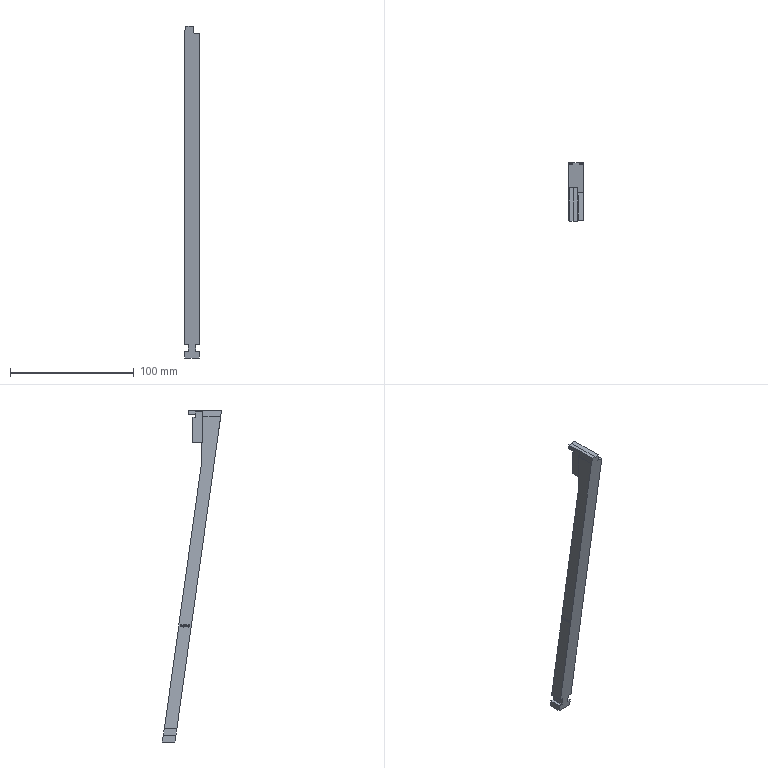Part | Creo | 1 solid | 123 faces | box 12 x 47.744 x 267.86 mm | volume 35156 mm3 | other 67 | plane 49 | cylinder 7 | commonest cylinder face diameters 1 x4 1.552 x1 2 x1 24.477 x1